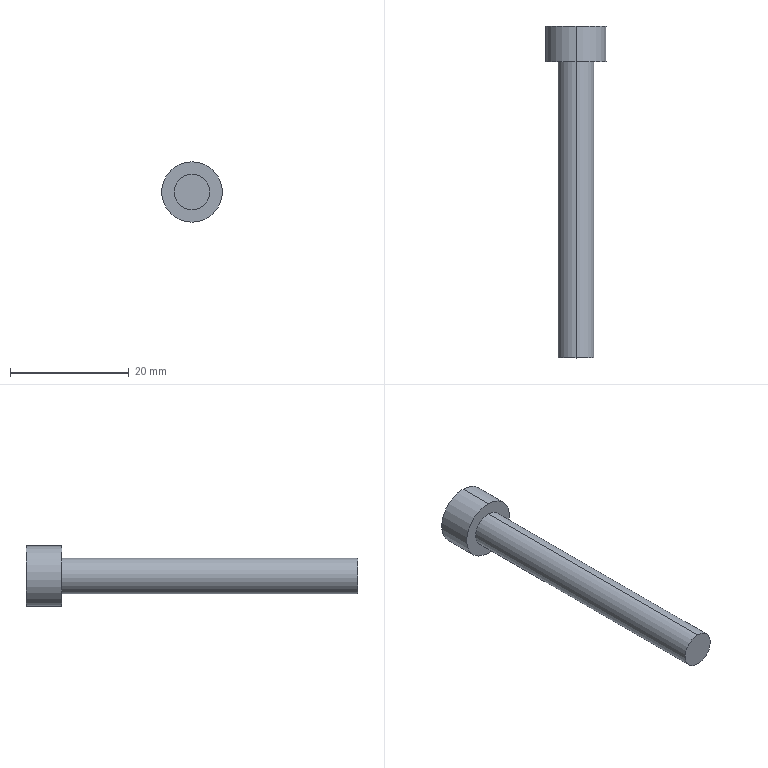Part | SolidWorks | features ICE 1, Revolution 1 | 1 solid | 14 faces | box 10.2 x 56 x 10.2 mm | volume 1796 mm3 | plane 10 | cylinder 4 | commonest cylinder face diameters 6 x2 10.2 x2
STEP:
#1=CARTESIAN_POINT('',(0.,-50.,3.));
#2=VERTEX_POINT('',#1);
#3=CARTESIAN_POINT('',(0.,-50.,-3.));
#4=VERTEX_POINT('',#3);
#5=CARTESIAN_POINT('',(0.,-50.,0.));
#6=DIRECTION('',(0.,1.,0.));
#7=DIRECTION('',(0.,0.,1.));
#8=AXIS2_PLACEMENT_3D('',#5,#6,#7);
#9=CIRCLE('',#8,3.);
#10=EDGE_CURVE('',#2,#4,#9,.T.);
#11=ORIENTED_EDGE('',*,*,#10,.T.);
#12=CARTESIAN_POINT('',(0.,0.,-3.));
#13=VERTEX_POINT('',#12);
#14=CARTESIAN_POINT('',(0.,11.322,-3.));
#15=DIRECTION('',(0.,1.,0.));
#16=VECTOR('',#15,1000.);
#17=LINE('',#14,#16);
#18=EDGE_CURVE('',#4,#13,#17,.T.);
#19=ORIENTED_EDGE('',*,*,#18,.T.);
#20=CARTESIAN_POINT('',(0.,0.,3.));
#21=VERTEX_POINT('',#20);
#22=CARTESIAN_POINT('',(0.,0.,0.));
#23=DIRECTION('',(0.,1.,0.));
#24=DIRECTION('',(0.,0.,1.));
#25=AXIS2_PLACEMENT_3D('',#22,#23,#24);
#26=CIRCLE('',#25,3.);
#27=EDGE_CURVE('',#21,#13,#26,.T.);
#28=ORIENTED_EDGE('',*,*,#27,.F.);
#29=CARTESIAN_POINT('',(0.,11.322,3.));
#30=DIRECTION('',(0.,1.,0.));
#31=VECTOR('',#30,1000.);
#32=LINE('',#29,#31);
#33=EDGE_CURVE('',#2,#21,#32,.T.);
#34=ORIENTED_EDGE('',*,*,#33,.F.);
#35=EDGE_LOOP('',(#11,#19,#28,#34));
#36=FACE_OUTER_BOUND('',#35,.T.);
#37=CARTESIAN_POINT('',(0.,11.322,0.));
#38=DIRECTION('',(0.,1.,0.));
#39=DIRECTION('',(0.,0.,1.));
#40=AXIS2_PLACEMENT_3D('',#37,#38,#39);
#41=CYLINDRICAL_SURFACE('',#40,3.);
#42=ADVANCED_FACE('',(#36),#41,.T.);
#43=CARTESIAN_POINT('',(0.,0.,5.1));
#44=VERTEX_POINT('',#43);
#45=CARTESIAN_POINT('',(0.,0.,-5.1));
#46=VERTEX_POINT('',#45);
#47=CARTESIAN_POINT('',(0.,0.,0.));
#48=DIRECTION('',(0.,1.,0.));
#49=DIRECTION('',(0.,0.,1.));
#50=AXIS2_PLACEMENT_3D('',#47,#48,#49);
#51=CIRCLE('',#50,5.1);
#52=EDGE_CURVE('',#44,#46,#51,.T.);
#53=ORIENTED_EDGE('',*,*,#52,.T.);
#54=CARTESIAN_POINT('',(0.,6.,-5.1));
#55=VERTEX_POINT('',#54);
#56=CARTESIAN_POINT('',(0.,11.322,-5.1));
#57=DIRECTION('',(0.,1.,0.));
#58=VECTOR('',#57,1000.);
#59=LINE('',#56,#58);
#60=EDGE_CURVE('',#46,#55,#59,.T.);
#61=ORIENTED_EDGE('',*,*,#60,.T.);
#62=CARTESIAN_POINT('',(0.,6.,5.1));
#63=VERTEX_POINT('',#62);
#64=CARTESIAN_POINT('',(0.,6.,0.));
#65=DIRECTION('',(0.,1.,0.));
#66=DIRECTION('',(0.,0.,1.));
#67=AXIS2_PLACEMENT_3D('',#64,#65,#66);
#68=CIRCLE('',#67,5.1);
#69=EDGE_CURVE('',#63,#55,#68,.T.);
#70=ORIENTED_EDGE('',*,*,#69,.F.);
#71=CARTESIAN_POINT('',(0.,11.322,5.1));
#72=DIRECTION('',(0.,1.,0.));
#73=VECTOR('',#72,1000.);
#74=LINE('',#71,#73);
#75=EDGE_CURVE('',#44,#63,#74,.T.);
#76=ORIENTED_EDGE('',*,*,#75,.F.);
#77=EDGE_LOOP('',(#53,#61,#70,#76));
#78=FACE_OUTER_BOUND('',#77,.T.);
#79=CARTESIAN_POINT('',(0.,11.322,0.));
#80=DIRECTION('',(0.,1.,0.));
#81=DIRECTION('',(0.,0.,1.));
#82=AXIS2_PLACEMENT_3D('',#79,#80,#81);
#83=CYLINDRICAL_SURFACE('',#82,5.1);
#84=ADVANCED_FACE('',(#78),#83,.T.);
#85=CARTESIAN_POINT('',(2.5,6.,-1.443));
#86=VERTEX_POINT('',#85);
#87=CARTESIAN_POINT('',(0.,6.,-2.887));
#88=VERTEX_POINT('',#87);
#89=CARTESIAN_POINT('',(2.5,6.,-1.443));
#90=DIRECTION('',(-0.866,0.,-0.5));
#91=VECTOR('',#90,1000.);
#92=LINE('',#89,#91);
#93=EDGE_CURVE('',#86,#88,#92,.T.);
#94=ORIENTED_EDGE('',*,*,#93,.F.);
#95=CARTESIAN_POINT('',(2.5,6.,1.443));
#96=VERTEX_POINT('',#95);
#97=CARTESIAN_POINT('',(2.5,6.,1.443));
#98=DIRECTION('',(0.,0.,-1.));
#99=VECTOR('',#98,1000.);
#100=LINE('',#97,#99);
#101=EDGE_CURVE('',#96,#86,#100,.T.);
#102=ORIENTED_EDGE('',*,*,#101,.F.);
#103=CARTESIAN_POINT('',(0.,6.,2.887));
#104=VERTEX_POINT('',#103);
#105=CARTESIAN_POINT('',(0.,6.,2.887));
#106=DIRECTION('',(0.866,0.,-0.5));
#107=VECTOR('',#106,1000.);
#108=LINE('',#105,#107);
#109=EDGE_CURVE('',#104,#96,#108,.T.);
#110=ORIENTED_EDGE('',*,*,#109,.F.);
#111=CARTESIAN_POINT('',(-2.5,6.,1.443));
#112=VERTEX_POINT('',#111);
#113=CARTESIAN_POINT('',(-2.5,6.,1.443));
#114=DIRECTION('',(0.866,0.,0.5));
#115=VECTOR('',#114,1000.);
#116=LINE('',#113,#115);
#117=EDGE_CURVE('',#112,#104,#116,.T.);
#118=ORIENTED_EDGE('',*,*,#117,.F.);
#119=CARTESIAN_POINT('',(-2.5,6.,-1.443));
#120=VERTEX_POINT('',#119);
#121=CARTESIAN_POINT('',(-2.5,6.,-1.443));
#122=DIRECTION('',(0.,0.,1.));
#123=VECTOR('',#122,1000.);
#124=LINE('',#121,#123);
#125=EDGE_CURVE('',#120,#112,#124,.T.);
#126=ORIENTED_EDGE('',*,*,#125,.F.);
#127=CARTESIAN_POINT('',(0.,6.,-2.887));
#128=DIRECTION('',(-0.866,0.,0.5));
#129=VECTOR('',#128,1000.);
#130=LINE('',#127,#129);
#131=EDGE_CURVE('',#88,#120,#130,.T.);
#132=ORIENTED_EDGE('',*,*,#131,.F.);
#133=EDGE_LOOP('',(#94,#102,#110,#118,#126,#132));
#134=FACE_BOUND('',#133,.T.);
#135=ORIENTED_EDGE('',*,*,#69,.T.);
#136=CARTESIAN_POINT('',(0.,6.,0.));
#137=DIRECTION('',(0.,1.,0.));
#138=DIRECTION('',(0.,0.,1.));
#139=AXIS2_PLACEMENT_3D('',#136,#137,#138);
#140=CIRCLE('',#139,5.1);
#141=EDGE_CURVE('',#55,#63,#140,.T.);
#142=ORIENTED_EDGE('',*,*,#141,.T.);
#143=EDGE_LOOP('',(#135,#142));
#144=FACE_OUTER_BOUND('',#143,.T.);
#145=CARTESIAN_POINT('',(0.,6.,0.));
#146=DIRECTION('',(0.,1.,0.));
#147=DIRECTION('',(0.,0.,1.));
#148=AXIS2_PLACEMENT_3D('',#145,#146,#147);
#149=PLANE('',#148);
#150=ADVANCED_FACE('',(#134,#144),#149,.T.);
#151=ORIENTED_EDGE('',*,*,#60,.F.);
#152=CARTESIAN_POINT('',(0.,0.,0.));
#153=DIRECTION('',(0.,1.,0.));
#154=DIRECTION('',(0.,0.,1.));
#155=AXIS2_PLACEMENT_3D('',#152,#153,#154);
#156=CIRCLE('',#155,5.1);
#157=EDGE_CURVE('',#46,#44,#156,.T.);
#158=ORIENTED_EDGE('',*,*,#157,.T.);
#159=ORIENTED_EDGE('',*,*,#75,.T.);
#160=ORIENTED_EDGE('',*,*,#141,.F.);
#161=EDGE_LOOP('',(#151,#158,#159,#160));
#162=FACE_OUTER_BOUND('',#161,.T.);
#163=CARTESIAN_POINT('',(0.,11.322,0.));
#164=DIRECTION('',(0.,1.,0.));
#165=DIRECTION('',(0.,0.,1.));
#166=AXIS2_PLACEMENT_3D('',#163,#164,#165);
#167=CYLINDRICAL_SURFACE('',#166,5.1);
#168=ADVANCED_FACE('',(#162),#167,.T.);
#169=ORIENTED_EDGE('',*,*,#27,.T.);
#170=CARTESIAN_POINT('',(0.,0.,0.));
#171=DIRECTION('',(0.,1.,0.));
#172=DIRECTION('',(0.,0.,1.));
#173=AXIS2_PLACEMENT_3D('',#170,#171,#172);
#174=CIRCLE('',#173,3.);
#175=EDGE_CURVE('',#13,#21,#174,.T.);
#176=ORIENTED_EDGE('',*,*,#175,.T.);
#177=EDGE_LOOP('',(#169,#176));
#178=FACE_BOUND('',#177,.T.);
#179=ORIENTED_EDGE('',*,*,#52,.F.);
#180=ORIENTED_EDGE('',*,*,#157,.F.);
#181=EDGE_LOOP('',(#179,#180));
#182=FACE_OUTER_BOUND('',#181,.T.);
#183=CARTESIAN_POINT('',(-5.1,0.,0.));
#184=DIRECTION('',(0.,-1.,0.));
#185=DIRECTION('',(0.,0.,-1.));
#186=AXIS2_PLACEMENT_3D('',#183,#184,#185);
#187=PLANE('',#186);
#188=ADVANCED_FACE('',(#178,#182),#187,.T.);
#189=ORIENTED_EDGE('',*,*,#18,.F.);
#190=CARTESIAN_POINT('',(0.,-50.,0.));
#191=DIRECTION('',(0.,1.,0.));
#192=DIRECTION('',(0.,0.,1.));
#193=AXIS2_PLACEMENT_3D('',#190,#191,#192);
#194=CIRCLE('',#193,3.);
#195=EDGE_CURVE('',#4,#2,#194,.T.);
#196=ORIENTED_EDGE('',*,*,#195,.T.);
#197=ORIENTED_EDGE('',*,*,#33,.T.);
#198=ORIENTED_EDGE('',*,*,#175,.F.);
#199=EDGE_LOOP('',(#189,#196,#197,#198));
#200=FACE_OUTER_BOUND('',#199,.T.);
#201=CARTESIAN_POINT('',(0.,11.322,0.));
#202=DIRECTION('',(0.,1.,0.));
#203=DIRECTION('',(0.,0.,1.));
#204=AXIS2_PLACEMENT_3D('',#201,#202,#203);
#205=CYLINDRICAL_SURFACE('',#204,3.);
#206=ADVANCED_FACE('',(#200),#205,.T.);
#207=ORIENTED_EDGE('',*,*,#10,.F.);
#208=ORIENTED_EDGE('',*,*,#195,.F.);
#209=EDGE_LOOP('',(#207,#208));
#210=FACE_OUTER_BOUND('',#209,.T.);
#211=CARTESIAN_POINT('',(-3.,-50.,0.));
#212=DIRECTION('',(0.,-1.,0.));
#213=DIRECTION('',(0.,0.,-1.));
#214=AXIS2_PLACEMENT_3D('',#211,#212,#213);
#215=PLANE('',#214);
#216=ADVANCED_FACE('',(#210),#215,.T.);
#217=ORIENTED_EDGE('',*,*,#93,.T.);
#218=CARTESIAN_POINT('',(0.,1.,-2.887));
#219=VERTEX_POINT('',#218);
#220=CARTESIAN_POINT('',(0.,1.,-2.887));
#221=DIRECTION('',(0.,1.,0.));
#222=VECTOR('',#221,1000.);
#223=LINE('',#220,#222);
#224=EDGE_CURVE('',#219,#88,#223,.T.);
#225=ORIENTED_EDGE('',*,*,#224,.F.);
#226=CARTESIAN_POINT('',(2.5,1.,-1.443));
#227=VERTEX_POINT('',#226);
#228=CARTESIAN_POINT('',(2.5,1.,-1.443));
#229=DIRECTION('',(-0.866,0.,-0.5));
#230=VECTOR('',#229,1000.);
#231=LINE('',#228,#230);
#232=EDGE_CURVE('',#227,#219,#231,.T.);
#233=ORIENTED_EDGE('',*,*,#232,.F.);
#234=CARTESIAN_POINT('',(2.5,1.,-1.443));
#235=DIRECTION('',(0.,1.,0.));
#236=VECTOR('',#235,1000.);
#237=LINE('',#234,#236);
#238=EDGE_CURVE('',#227,#86,#237,.T.);
#239=ORIENTED_EDGE('',*,*,#238,.T.);
#240=EDGE_LOOP('',(#217,#225,#233,#239));
#241=FACE_OUTER_BOUND('',#240,.T.);
#242=CARTESIAN_POINT('',(2.5,1.,-1.443));
#243=DIRECTION('',(0.5,0.,-0.866));
#244=DIRECTION('',(-0.866,0.,-0.5));
#245=AXIS2_PLACEMENT_3D('',#242,#243,#244);
#246=PLANE('',#245);
#247=ADVANCED_FACE('',(#241),#246,.F.);
#248=ORIENTED_EDGE('',*,*,#101,.T.);
#249=ORIENTED_EDGE('',*,*,#238,.F.);
#250=CARTESIAN_POINT('',(2.5,1.,1.443));
#251=VERTEX_POINT('',#250);
#252=CARTESIAN_POINT('',(2.5,1.,1.443));
#253=DIRECTION('',(0.,0.,-1.));
#254=VECTOR('',#253,1000.);
#255=LINE('',#252,#254);
#256=EDGE_CURVE('',#251,#227,#255,.T.);
#257=ORIENTED_EDGE('',*,*,#256,.F.);
#258=CARTESIAN_POINT('',(2.5,1.,1.443));
#259=DIRECTION('',(0.,1.,0.));
#260=VECTOR('',#259,1000.);
#261=LINE('',#258,#260);
#262=EDGE_CURVE('',#251,#96,#261,.T.);
#263=ORIENTED_EDGE('',*,*,#262,.T.);
#264=EDGE_LOOP('',(#248,#249,#257,#263));
#265=FACE_OUTER_BOUND('',#264,.T.);
#266=CARTESIAN_POINT('',(2.5,1.,1.443));
#267=DIRECTION('',(1.,0.,0.));
#268=DIRECTION('',(0.,0.,-1.));
#269=AXIS2_PLACEMENT_3D('',#266,#267,#268);
#270=PLANE('',#269);
#271=ADVANCED_FACE('',(#265),#270,.F.);
#272=ORIENTED_EDGE('',*,*,#109,.T.);
#273=ORIENTED_EDGE('',*,*,#262,.F.);
#274=CARTESIAN_POINT('',(0.,1.,2.887));
#275=VERTEX_POINT('',#274);
#276=CARTESIAN_POINT('',(0.,1.,2.887));
#277=DIRECTION('',(0.866,0.,-0.5));
#278=VECTOR('',#277,1000.);
#279=LINE('',#276,#278);
#280=EDGE_CURVE('',#275,#251,#279,.T.);
#281=ORIENTED_EDGE('',*,*,#280,.F.);
#282=CARTESIAN_POINT('',(0.,1.,2.887));
#283=DIRECTION('',(0.,1.,0.));
#284=VECTOR('',#283,1000.);
#285=LINE('',#282,#284);
#286=EDGE_CURVE('',#275,#104,#285,.T.);
#287=ORIENTED_EDGE('',*,*,#286,.T.);
#288=EDGE_LOOP('',(#272,#273,#281,#287));
#289=FACE_OUTER_BOUND('',#288,.T.);
#290=CARTESIAN_POINT('',(0.,1.,2.887));
#291=DIRECTION('',(0.5,0.,0.866));
#292=DIRECTION('',(0.866,0.,-0.5));
#293=AXIS2_PLACEMENT_3D('',#290,#291,#292);
#294=PLANE('',#293);
#295=ADVANCED_FACE('',(#289),#294,.F.);
#296=ORIENTED_EDGE('',*,*,#117,.T.);
#297=ORIENTED_EDGE('',*,*,#286,.F.);
#298=CARTESIAN_POINT('',(-2.5,1.,1.443));
#299=VERTEX_POINT('',#298);
#300=CARTESIAN_POINT('',(-2.5,1.,1.443));
#301=DIRECTION('',(0.866,0.,0.5));
#302=VECTOR('',#301,1000.);
#303=LINE('',#300,#302);
#304=EDGE_CURVE('',#299,#275,#303,.T.);
#305=ORIENTED_EDGE('',*,*,#304,.F.);
#306=CARTESIAN_POINT('',(-2.5,1.,1.443));
#307=DIRECTION('',(0.,1.,0.));
#308=VECTOR('',#307,1000.);
#309=LINE('',#306,#308);
#310=EDGE_CURVE('',#299,#112,#309,.T.);
#311=ORIENTED_EDGE('',*,*,#310,.T.);
#312=EDGE_LOOP('',(#296,#297,#305,#311));
#313=FACE_OUTER_BOUND('',#312,.T.);
#314=CARTESIAN_POINT('',(-2.5,1.,1.443));
#315=DIRECTION('',(-0.5,0.,0.866));
#316=DIRECTION('',(0.866,0.,0.5));
#317=AXIS2_PLACEMENT_3D('',#314,#315,#316);
#318=PLANE('',#317);
#319=ADVANCED_FACE('',(#313),#318,.F.);
#320=ORIENTED_EDGE('',*,*,#125,.T.);
#321=ORIENTED_EDGE('',*,*,#310,.F.);
#322=CARTESIAN_POINT('',(-2.5,1.,-1.443));
#323=VERTEX_POINT('',#322);
#324=CARTESIAN_POINT('',(-2.5,1.,-1.443));
#325=DIRECTION('',(0.,0.,1.));
#326=VECTOR('',#325,1000.);
#327=LINE('',#324,#326);
#328=EDGE_CURVE('',#323,#299,#327,.T.);
#329=ORIENTED_EDGE('',*,*,#328,.F.);
#330=CARTESIAN_POINT('',(-2.5,1.,-1.443));
#331=DIRECTION('',(0.,1.,0.));
#332=VECTOR('',#331,1000.);
#333=LINE('',#330,#332);
#334=EDGE_CURVE('',#323,#120,#333,.T.);
#335=ORIENTED_EDGE('',*,*,#334,.T.);
#336=EDGE_LOOP('',(#320,#321,#329,#335));
#337=FACE_OUTER_BOUND('',#336,.T.);
#338=CARTESIAN_POINT('',(-2.5,1.,-1.443));
#339=DIRECTION('',(-1.,0.,0.));
#340=DIRECTION('',(0.,0.,1.));
#341=AXIS2_PLACEMENT_3D('',#338,#339,#340);
#342=PLANE('',#341);
#343=ADVANCED_FACE('',(#337),#342,.F.);
#344=ORIENTED_EDGE('',*,*,#131,.T.);
#345=ORIENTED_EDGE('',*,*,#334,.F.);
#346=CARTESIAN_POINT('',(0.,1.,-2.887));
#347=DIRECTION('',(-0.866,0.,0.5));
#348=VECTOR('',#347,1000.);
#349=LINE('',#346,#348);
#350=EDGE_CURVE('',#219,#323,#349,.T.);
#351=ORIENTED_EDGE('',*,*,#350,.F.);
#352=ORIENTED_EDGE('',*,*,#224,.T.);
#353=EDGE_LOOP('',(#344,#345,#351,#352));
#354=FACE_OUTER_BOUND('',#353,.T.);
#355=CARTESIAN_POINT('',(0.,1.,-2.887));
#356=DIRECTION('',(-0.5,0.,-0.866));
#357=DIRECTION('',(-0.866,0.,0.5));
#358=AXIS2_PLACEMENT_3D('',#355,#356,#357);
#359=PLANE('',#358);
#360=ADVANCED_FACE('',(#354),#359,.F.);
#361=ORIENTED_EDGE('',*,*,#232,.T.);
#362=ORIENTED_EDGE('',*,*,#350,.T.);
#363=ORIENTED_EDGE('',*,*,#328,.T.);
#364=ORIENTED_EDGE('',*,*,#304,.T.);
#365=ORIENTED_EDGE('',*,*,#280,.T.);
#366=ORIENTED_EDGE('',*,*,#256,.T.);
#367=EDGE_LOOP('',(#361,#362,#363,#364,#365,#366));
#368=FACE_OUTER_BOUND('',#367,.T.);
#369=CARTESIAN_POINT('',(0.,1.,0.));
#370=DIRECTION('',(0.,1.,0.));
#371=DIRECTION('',(0.,0.,1.));
#372=AXIS2_PLACEMENT_3D('',#369,#370,#371);
#373=PLANE('',#372);
#374=ADVANCED_FACE('',(#368),#373,.T.);
#375=CLOSED_SHELL('',(#42,#84,#150,#168,#188,#206,#216,#247,#271,#295,#319,#343,#360,#374));
#376=MANIFOLD_SOLID_BREP('',#375);
#377=CARTESIAN_POINT('',(0.,0.,0.));
#378=DIRECTION('',(0.,0.,1.));
#379=DIRECTION('',(1.,0.,0.));
#380=AXIS2_PLACEMENT_3D('',#377,#378,#379);
#381=(LENGTH_UNIT()NAMED_UNIT(*)SI_UNIT(.MILLI.,.METRE.));
#382=UNCERTAINTY_MEASURE_WITH_UNIT(LENGTH_MEASURE(0.00001),#381,'','');
#383=(NAMED_UNIT(*)PLANE_ANGLE_UNIT()SI_UNIT($,.RADIAN.));
#384=(NAMED_UNIT(*)SI_UNIT($,.STERADIAN.)SOLID_ANGLE_UNIT());
#385=(GEOMETRIC_REPRESENTATION_CONTEXT(3)GLOBAL_UNCERTAINTY_ASSIGNED_CONTEXT((#382))GLOBAL_UNIT_ASSIGNED_CONTEXT((#381,#383,#384))REPRESENTATION_CONTEXT('',''));
#386=ADVANCED_BREP_SHAPE_REPRESENTATION('',(#376,#380),#385);